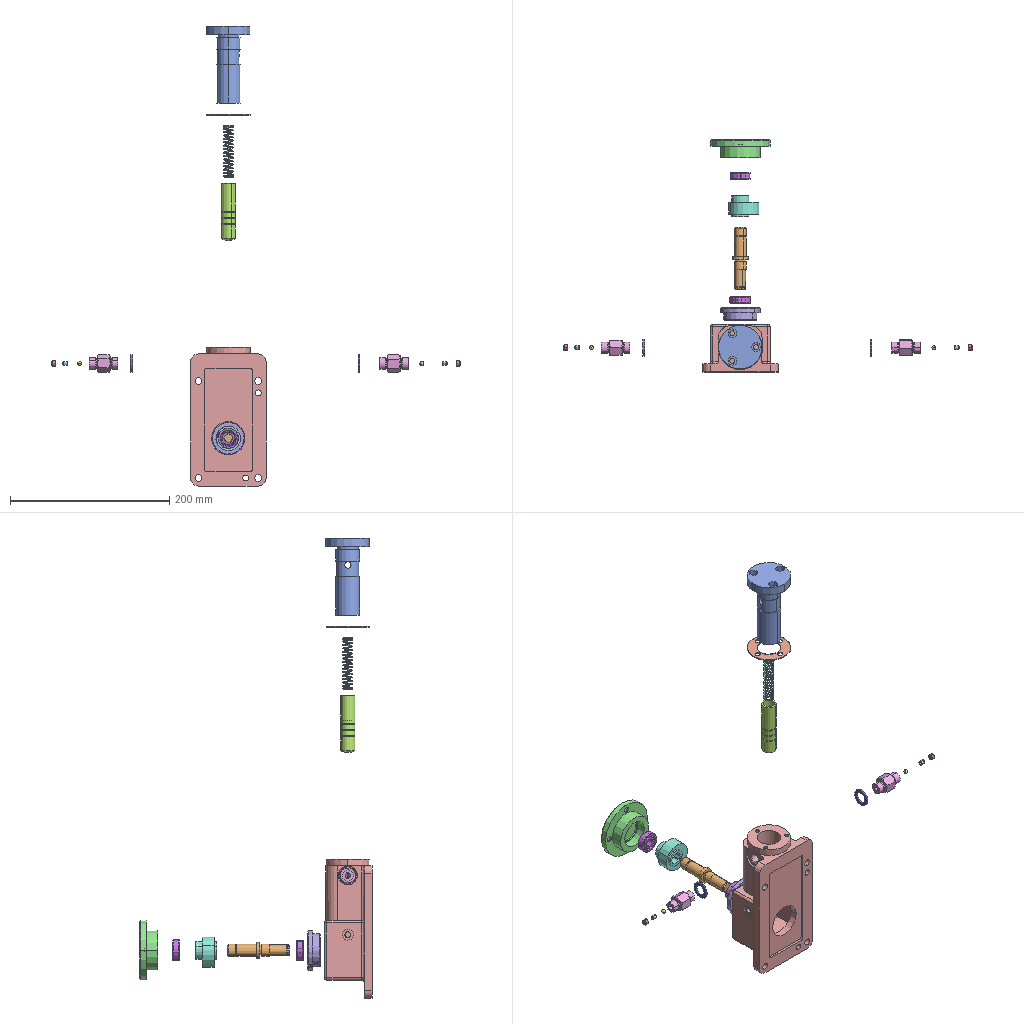Assembly | SolidWorks | 21 different items | 27 placed | box 514 x 292 x 578 mm
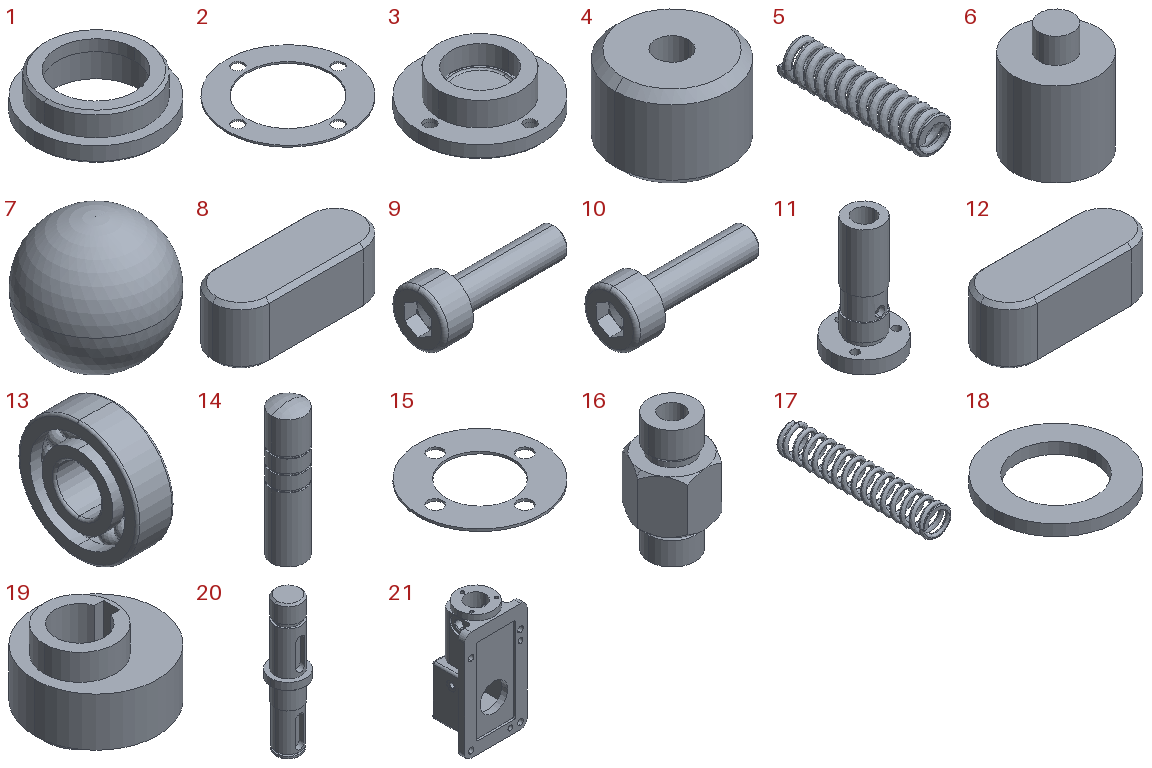Parts list (item | quantity | size | volume | features):
1 | x1 | 50 x 50 x 15.5 mm | 11056 mm3 | features ICE 4, Chamfer 1, Extrusion 1
2 | x1 | 75 x 75 x 1 mm | 2300 mm3 | features Extrusion 1
3 | x1 | 75 x 75 x 22.5 mm | 47960 mm3 | features ICE 7, Chamfer 1, CirPattern 1, Extrusion 1, Fillet 1
4 | x2 | 7 x 7 x 5 mm | 171.479 mm3 | features Chamfer 1, Extrusion 1, ICE 1
5 | x1 | - | 136.283 mm3 | features Sweep 3, ICE 1
6 | x2 | 5 x 5 x 6.5 mm | 79.849 mm3 | features Extrusion 1, ICE 1, RevCut 1
7 | x2 | 5 x 5 x 5 mm | 65.45 mm3 | features Revolution 1
8 | x1 | 8 x 3 x 3 mm | 65.446 mm3 | features Boss 2, Chamfer 1, Extrusion 1
9 | x1 | 7.6 x 3 x 3 mm | 21.652 mm3 | features Fillet 2, RevCut 2, Boss 1, Chamfer 1, Cut 1, Extrusion 1, LPattern 1
10 | x1 | 7.6 x 3 x 3 mm | 21.652 mm3 | features Fillet 2, RevCut 2, Boss 1, Chamfer 1, Cut 1, Extrusion 1, LPattern 1
11 | x1 | 55 x 55 x 97 mm | 56843 mm3 | features ICE 9, CirPattern 1, Extrusion 1
12 | x1 | 8 x 3 x 3 mm | 65.446 mm3 | features Boss 2, Chamfer 1, Extrusion 1
13 | x2 | 8 x 26 x 26 mm | 2684 mm3 | features Revolution 3, CirPattern 1, Fillet 1
14 | x1 | 18 x 18 x 71.992 mm | 12874 mm3 | features ICE 4, Extrusion 1, HoleWzd 1, Revolution 1
15 | x1 | 55 x 55 x 1 mm | 1536 mm3 | features Extrusion 1
16 | x2 | 21.906 x 19.575 x 36 mm | 6912 mm3 | features ICE 4, RevCut 2, StudWizard 2, Extrusion 1
17 | x1 | - | 1390 mm3 | features Sweep 3, ICE 1
18 | x2 | 22 x 22 x 2 mm | 452.389 mm3 | features Extrusion 1
19 | x1 | 38 x 38 x 26 mm | 16281 mm3 | features ICE 2, Extrusion 1
20 | x1 | 20 x 20 x 78 mm | 13019 mm3 | features ICE 10, Chamfer 1, Extrusion 1
21 | x1 | 95 x 59.897 x 174.5 mm | 358133 mm3 | features ICE 17, Fillet 4, HoleWzd 4, CirPattern 1, Extrusion 1, MirrorPattern 1
Mates (type | each side: item.copy, entity, surface, feature):
Coincident | 11.1 face plane Cut-Extrude2 | 17.1 face plane Cut-Extrude1
Lock | 11.1 select_type:0 | 17.1 select_type:0
Concentric | 11.1 face cylinder Boss-Extrude5 | 14.1 face cylinder Boss-Extrude1
Coincident | 14.1 face plane Cut-Extrude1 | 17.1 face plane Cut-Extrude1
Concentric | 21.1 face cylinder Cut-Extrude1 | 11.1 face cylinder Boss-Extrude5
Concentric | 21.1 edge | 11.1 face cylinder Cut-Extrude5
Concentric | 11.1 face cylinder Boss-Extrude1 | 15.1 edge
Coincident | 11.1 face plane Boss-Extrude1 | 15.1 face plane Boss-Extrude1
Concentric | 21.1 edge | 18.1 edge
Coincident | 21.1 face plane Mirror1 | 18.1 face plane Boss-Extrude1
Concentric | 21.1 face cone Mirror1 | 16.1 face cylinder Boss-Extrude1
Coincident | 16.1 face plane Boss-Extrude3 | 18.1 face plane Boss-Extrude1
Concentric | 21.1 face cylinder Cut-Extrude10 | 18.2 edge
Coincident | 21.1 face plane Cut-Extrude10 | 18.2 face plane Boss-Extrude1
Concentric | 21.1 face cylinder Cut-Extrude10 | 16.2 face cylinder Boss-Extrude1
Coincident | 16.2 face plane Boss-Extrude3 | 18.2 face plane Boss-Extrude1
Concentric | 21.1 face cylinder Cut-Extrude7 | 1.1 face cylinder Boss-Extrude3
Coincident | 21.1 face plane Boss-Extrude6 | 1.1 face plane Boss-Extrude1
Concentric | 1.1 face cylinder Cut-Extrude3 | 13.1 face cylinder Revolve3
Concentric | 20.1 face cylinder Boss-Extrude4 | 13.1 face cylinder Revolve3
Coincident | 20.1 face plane Boss-Extrude6 | 13.1 face plane Revolve2
Concentric | 20.1 face cylinder Boss-Extrude9 | 13.2 edge
Coincident | 20.1 face plane Boss-Extrude9 | 13.2 face plane Revolve2
Concentric | 19.1 face cylinder Cut-Extrude1 | 20.1 face cylinder Boss-Extrude7
Parallel | 19.1 face plane Cut-Extrude1 | 20.1 face plane Cut-Extrude2
Coincident | 19.1 face plane Boss-Extrude1 | 20.1 face plane Boss-Extrude6
Coincident | 1.1 face plane Cut-Extrude3 | 13.1 face plane Revolve3
Concentric | 21.1 face cylinder Cut-Extrude2 | 3.1 face cylinder Boss-Extrude2
Coincident | 21.1 face plane Boss-Extrude2 | 3.1 face plane Boss-Extrude1
Concentric | 21.1 face cylinder M6 Tapped Hole1 | 3.1 face cylinder CirPattern1
Concentric | 6.1 face sphere Cut-Revolve1 | 7.1 face sphere Revolve1
Concentric | 16.1 face cylinder Cut-Revolve3 | 6.1 face cylinder Boss-Extrude1
Tangent | 16.1 face sphere Cut-Revolve3 | 7.1 face sphere Revolve1
Tangent | 7.2 face sphere Revolve1 | 6.2 face sphere Cut-Revolve1
Concentric | 16.2 face cylinder Cut-Revolve3 | 6.2 face cylinder Boss-Extrude1
Concentric | 16.2 face sphere Cut-Revolve3 | 7.2 face sphere Revolve1
Concentric | 16.2 face cylinder Cut-Revolve3 | 4.1 face cylinder Boss-Extrude1
Coincident | 16.2 face plane Boss-Extrude5 | 4.1 face plane Boss-Extrude1
Concentric | 16.1 edge | 4.2 face cylinder Boss-Extrude1
Coincident | 16.1 face plane Boss-Extrude5 | 4.2 face plane Boss-Extrude1